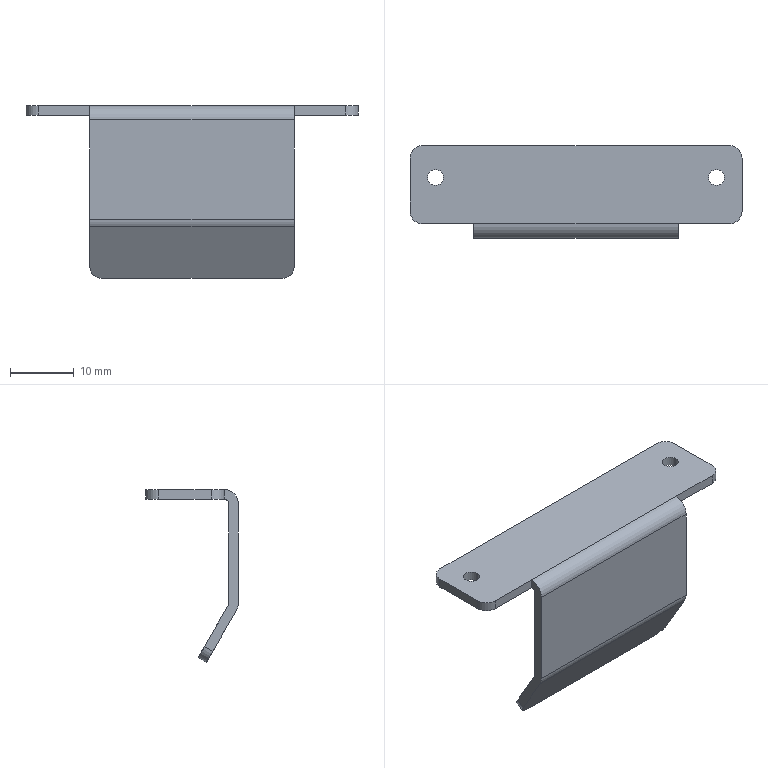Part | STEP file | 06-01-10 light source inclined plate A (Default) | 1 solid | 28 faces | box 52 x 14.5 x 27.062 mm | volume 2282 mm3 | cylinder 14 | plane 14 | commonest cylinder face diameters 4 x6 2.5 x4 1.473 x2 4.473 x2
STEP:
#1=CARTESIAN_POINT('',(20.75,1.5,0.));
#2=VERTEX_POINT('',#1);
#3=CARTESIAN_POINT('',(23.25,1.5,0.));
#4=VERTEX_POINT('',#3);
#5=CARTESIAN_POINT('',(22.,1.5,0.));
#6=DIRECTION('',(0.,0.,1.));
#7=DIRECTION('',(1.,0.,0.));
#8=AXIS2_PLACEMENT_3D('',#5,#6,#7);
#9=CIRCLE('',#8,1.25);
#10=EDGE_CURVE('',#2,#4,#9,.T.);
#11=ORIENTED_EDGE('',*,*,#10,.T.);
#12=CARTESIAN_POINT('',(23.25,1.5,-1.5));
#13=VERTEX_POINT('',#12);
#14=CARTESIAN_POINT('',(23.25,1.5,-1.5));
#15=DIRECTION('',(0.,0.,-1.));
#16=VECTOR('',#15,1000.);
#17=LINE('',#14,#16);
#18=EDGE_CURVE('',#4,#13,#17,.T.);
#19=ORIENTED_EDGE('',*,*,#18,.T.);
#20=CARTESIAN_POINT('',(20.75,1.5,-1.5));
#21=VERTEX_POINT('',#20);
#22=CARTESIAN_POINT('',(22.,1.5,-1.5));
#23=DIRECTION('',(0.,0.,-1.));
#24=DIRECTION('',(-1.,0.,0.));
#25=AXIS2_PLACEMENT_3D('',#22,#23,#24);
#26=CIRCLE('',#25,1.25);
#27=EDGE_CURVE('',#13,#21,#26,.T.);
#28=ORIENTED_EDGE('',*,*,#27,.T.);
#29=CARTESIAN_POINT('',(20.75,1.5,-1.5));
#30=DIRECTION('',(0.,0.,-1.));
#31=VECTOR('',#30,1000.);
#32=LINE('',#29,#31);
#33=EDGE_CURVE('',#2,#21,#32,.T.);
#34=ORIENTED_EDGE('',*,*,#33,.F.);
#35=EDGE_LOOP('',(#11,#19,#28,#34));
#36=FACE_OUTER_BOUND('',#35,.T.);
#37=CARTESIAN_POINT('',(22.,1.5,-1.5));
#38=DIRECTION('',(0.,0.,-1.));
#39=DIRECTION('',(-1.,0.,0.));
#40=AXIS2_PLACEMENT_3D('',#37,#38,#39);
#41=CYLINDRICAL_SURFACE('',#40,1.25);
#42=ADVANCED_FACE('',(#36),#41,.F.);
#43=CARTESIAN_POINT('',(-23.25,1.5,0.));
#44=VERTEX_POINT('',#43);
#45=CARTESIAN_POINT('',(-20.75,1.5,0.));
#46=VERTEX_POINT('',#45);
#47=CARTESIAN_POINT('',(-22.,1.5,0.));
#48=DIRECTION('',(0.,0.,1.));
#49=DIRECTION('',(1.,0.,0.));
#50=AXIS2_PLACEMENT_3D('',#47,#48,#49);
#51=CIRCLE('',#50,1.25);
#52=EDGE_CURVE('',#44,#46,#51,.T.);
#53=ORIENTED_EDGE('',*,*,#52,.T.);
#54=CARTESIAN_POINT('',(-20.75,1.5,-1.5));
#55=VERTEX_POINT('',#54);
#56=CARTESIAN_POINT('',(-20.75,1.5,-1.5));
#57=DIRECTION('',(0.,0.,-1.));
#58=VECTOR('',#57,1000.);
#59=LINE('',#56,#58);
#60=EDGE_CURVE('',#46,#55,#59,.T.);
#61=ORIENTED_EDGE('',*,*,#60,.T.);
#62=CARTESIAN_POINT('',(-23.25,1.5,-1.5));
#63=VERTEX_POINT('',#62);
#64=CARTESIAN_POINT('',(-22.,1.5,-1.5));
#65=DIRECTION('',(0.,0.,-1.));
#66=DIRECTION('',(-1.,0.,0.));
#67=AXIS2_PLACEMENT_3D('',#64,#65,#66);
#68=CIRCLE('',#67,1.25);
#69=EDGE_CURVE('',#55,#63,#68,.T.);
#70=ORIENTED_EDGE('',*,*,#69,.T.);
#71=CARTESIAN_POINT('',(-23.25,1.5,-1.5));
#72=DIRECTION('',(0.,0.,-1.));
#73=VECTOR('',#72,1000.);
#74=LINE('',#71,#73);
#75=EDGE_CURVE('',#44,#63,#74,.T.);
#76=ORIENTED_EDGE('',*,*,#75,.F.);
#77=EDGE_LOOP('',(#53,#61,#70,#76));
#78=FACE_OUTER_BOUND('',#77,.T.);
#79=CARTESIAN_POINT('',(-22.,1.5,-1.5));
#80=DIRECTION('',(0.,0.,-1.));
#81=DIRECTION('',(-1.,0.,0.));
#82=AXIS2_PLACEMENT_3D('',#79,#80,#81);
#83=CYLINDRICAL_SURFACE('',#82,1.25);
#84=ADVANCED_FACE('',(#78),#83,.F.);
#85=CARTESIAN_POINT('',(16.,-8.,-2.237));
#86=VERTEX_POINT('',#85);
#87=CARTESIAN_POINT('',(16.,-8.,-17.803));
#88=VERTEX_POINT('',#87);
#89=CARTESIAN_POINT('',(16.,-8.,-1.5));
#90=DIRECTION('',(0.,0.,-1.));
#91=VECTOR('',#90,1000.);
#92=LINE('',#89,#91);
#93=EDGE_CURVE('',#86,#88,#92,.T.);
#94=ORIENTED_EDGE('',*,*,#93,.F.);
#95=CARTESIAN_POINT('',(-16.,-8.,-2.237));
#96=VERTEX_POINT('',#95);
#97=CARTESIAN_POINT('',(-26.,-8.,-2.237));
#98=DIRECTION('',(-1.,0.,0.));
#99=VECTOR('',#98,1000.);
#100=LINE('',#97,#99);
#101=EDGE_CURVE('',#86,#96,#100,.T.);
#102=ORIENTED_EDGE('',*,*,#101,.T.);
#103=CARTESIAN_POINT('',(-16.,-8.,-17.803));
#104=VERTEX_POINT('',#103);
#105=CARTESIAN_POINT('',(-16.,-8.,-1.5));
#106=DIRECTION('',(0.,0.,1.));
#107=VECTOR('',#106,1000.);
#108=LINE('',#105,#107);
#109=EDGE_CURVE('',#104,#96,#108,.T.);
#110=ORIENTED_EDGE('',*,*,#109,.F.);
#111=CARTESIAN_POINT('',(-26.,-8.,-17.803));
#112=DIRECTION('',(1.,0.,0.));
#113=VECTOR('',#112,1000.);
#114=LINE('',#111,#113);
#115=EDGE_CURVE('',#104,#88,#114,.T.);
#116=ORIENTED_EDGE('',*,*,#115,.T.);
#117=EDGE_LOOP('',(#94,#102,#110,#116));
#118=FACE_OUTER_BOUND('',#117,.T.);
#119=CARTESIAN_POINT('',(-26.,-8.,-1.5));
#120=DIRECTION('',(0.,-1.,0.));
#121=DIRECTION('',(0.,0.,-1.));
#122=AXIS2_PLACEMENT_3D('',#119,#120,#121);
#123=PLANE('',#122);
#124=ADVANCED_FACE('',(#118),#123,.T.);
#125=CARTESIAN_POINT('',(16.,-6.5,-2.237));
#126=VERTEX_POINT('',#125);
#127=CARTESIAN_POINT('',(-16.,-6.5,-2.237));
#128=VERTEX_POINT('',#127);
#129=CARTESIAN_POINT('',(26.,-6.5,-2.237));
#130=DIRECTION('',(-1.,0.,0.));
#131=VECTOR('',#130,1000.);
#132=LINE('',#129,#131);
#133=EDGE_CURVE('',#126,#128,#132,.T.);
#134=ORIENTED_EDGE('',*,*,#133,.F.);
#135=CARTESIAN_POINT('',(16.,-6.5,-17.803));
#136=VERTEX_POINT('',#135);
#137=CARTESIAN_POINT('',(16.,-6.5,-1.5));
#138=DIRECTION('',(0.,0.,-1.));
#139=VECTOR('',#138,1000.);
#140=LINE('',#137,#139);
#141=EDGE_CURVE('',#126,#136,#140,.T.);
#142=ORIENTED_EDGE('',*,*,#141,.T.);
#143=CARTESIAN_POINT('',(-16.,-6.5,-17.803));
#144=VERTEX_POINT('',#143);
#145=CARTESIAN_POINT('',(-26.,-6.5,-17.803));
#146=DIRECTION('',(1.,0.,0.));
#147=VECTOR('',#146,1000.);
#148=LINE('',#145,#147);
#149=EDGE_CURVE('',#144,#136,#148,.T.);
#150=ORIENTED_EDGE('',*,*,#149,.F.);
#151=CARTESIAN_POINT('',(-16.,-6.5,-1.5));
#152=DIRECTION('',(0.,0.,1.));
#153=VECTOR('',#152,1000.);
#154=LINE('',#151,#153);
#155=EDGE_CURVE('',#144,#128,#154,.T.);
#156=ORIENTED_EDGE('',*,*,#155,.T.);
#157=EDGE_LOOP('',(#134,#142,#150,#156));
#158=FACE_OUTER_BOUND('',#157,.T.);
#159=CARTESIAN_POINT('',(-26.,-6.5,-1.5));
#160=DIRECTION('',(0.,-1.,0.));
#161=DIRECTION('',(0.,0.,-1.));
#162=AXIS2_PLACEMENT_3D('',#159,#160,#161);
#163=PLANE('',#162);
#164=ADVANCED_FACE('',(#158),#163,.F.);
#165=CARTESIAN_POINT('',(-26.,4.5,-1.5));
#166=VERTEX_POINT('',#165);
#167=CARTESIAN_POINT('',(-26.,-3.763,-1.5));
#168=VERTEX_POINT('',#167);
#169=CARTESIAN_POINT('',(-26.,6.5,-1.5));
#170=DIRECTION('',(0.,-1.,0.));
#171=VECTOR('',#170,1000.);
#172=LINE('',#169,#171);
#173=EDGE_CURVE('',#166,#168,#172,.T.);
#174=ORIENTED_EDGE('',*,*,#173,.T.);
#175=CARTESIAN_POINT('',(-26.,-3.763,0.));
#176=VERTEX_POINT('',#175);
#177=CARTESIAN_POINT('',(-26.,-3.763,0.));
#178=DIRECTION('',(0.,0.,1.));
#179=VECTOR('',#178,1000.);
#180=LINE('',#177,#179);
#181=EDGE_CURVE('',#168,#176,#180,.T.);
#182=ORIENTED_EDGE('',*,*,#181,.T.);
#183=CARTESIAN_POINT('',(-26.,4.5,0.));
#184=VERTEX_POINT('',#183);
#185=CARTESIAN_POINT('',(-26.,6.5,0.));
#186=DIRECTION('',(0.,-1.,0.));
#187=VECTOR('',#186,1000.);
#188=LINE('',#185,#187);
#189=EDGE_CURVE('',#184,#176,#188,.T.);
#190=ORIENTED_EDGE('',*,*,#189,.F.);
#191=CARTESIAN_POINT('',(-26.,4.5,-1.5));
#192=DIRECTION('',(0.,0.,-1.));
#193=VECTOR('',#192,1000.);
#194=LINE('',#191,#193);
#195=EDGE_CURVE('',#184,#166,#194,.T.);
#196=ORIENTED_EDGE('',*,*,#195,.T.);
#197=EDGE_LOOP('',(#174,#182,#190,#196));
#198=FACE_OUTER_BOUND('',#197,.T.);
#199=CARTESIAN_POINT('',(-26.,6.5,-1.5));
#200=DIRECTION('',(-1.,0.,0.));
#201=DIRECTION('',(0.,0.,1.));
#202=AXIS2_PLACEMENT_3D('',#199,#200,#201);
#203=PLANE('',#202);
#204=ADVANCED_FACE('',(#198),#203,.T.);
#205=CARTESIAN_POINT('',(22.,1.5,-1.5));
#206=DIRECTION('',(0.,0.,-1.));
#207=DIRECTION('',(-1.,0.,0.));
#208=AXIS2_PLACEMENT_3D('',#205,#206,#207);
#209=CIRCLE('',#208,1.25);
#210=EDGE_CURVE('',#21,#13,#209,.T.);
#211=ORIENTED_EDGE('',*,*,#210,.F.);
#212=ORIENTED_EDGE('',*,*,#27,.F.);
#213=EDGE_LOOP('',(#211,#212));
#214=FACE_BOUND('',#213,.T.);
#215=CARTESIAN_POINT('',(-22.,1.5,-1.5));
#216=DIRECTION('',(0.,0.,-1.));
#217=DIRECTION('',(-1.,0.,0.));
#218=AXIS2_PLACEMENT_3D('',#215,#216,#217);
#219=CIRCLE('',#218,1.25);
#220=EDGE_CURVE('',#63,#55,#219,.T.);
#221=ORIENTED_EDGE('',*,*,#220,.F.);
#222=ORIENTED_EDGE('',*,*,#69,.F.);
#223=EDGE_LOOP('',(#221,#222));
#224=FACE_BOUND('',#223,.T.);
#225=CARTESIAN_POINT('',(-24.,-5.763,-1.5));
#226=VERTEX_POINT('',#225);
#227=CARTESIAN_POINT('',(-16.,-5.763,-1.5));
#228=VERTEX_POINT('',#227);
#229=CARTESIAN_POINT('',(-26.,-5.763,-1.5));
#230=DIRECTION('',(1.,0.,0.));
#231=VECTOR('',#230,1000.);
#232=LINE('',#229,#231);
#233=EDGE_CURVE('',#226,#228,#232,.T.);
#234=ORIENTED_EDGE('',*,*,#233,.F.);
#235=CARTESIAN_POINT('',(-24.,-3.763,-1.5));
#236=DIRECTION('',(0.,0.,-1.));
#237=DIRECTION('',(1.,0.,0.));
#238=AXIS2_PLACEMENT_3D('',#235,#236,#237);
#239=CIRCLE('',#238,2.);
#240=EDGE_CURVE('',#226,#168,#239,.T.);
#241=ORIENTED_EDGE('',*,*,#240,.T.);
#242=ORIENTED_EDGE('',*,*,#173,.F.);
#243=CARTESIAN_POINT('',(-24.,6.5,-1.5));
#244=VERTEX_POINT('',#243);
#245=CARTESIAN_POINT('',(-24.,4.5,-1.5));
#246=DIRECTION('',(0.,0.,-1.));
#247=DIRECTION('',(1.,0.,0.));
#248=AXIS2_PLACEMENT_3D('',#245,#246,#247);
#249=CIRCLE('',#248,2.);
#250=EDGE_CURVE('',#166,#244,#249,.T.);
#251=ORIENTED_EDGE('',*,*,#250,.T.);
#252=CARTESIAN_POINT('',(24.,6.5,-1.5));
#253=VERTEX_POINT('',#252);
#254=CARTESIAN_POINT('',(-26.,6.5,-1.5));
#255=DIRECTION('',(-1.,0.,0.));
#256=VECTOR('',#255,1000.);
#257=LINE('',#254,#256);
#258=EDGE_CURVE('',#253,#244,#257,.T.);
#259=ORIENTED_EDGE('',*,*,#258,.F.);
#260=CARTESIAN_POINT('',(26.,4.5,-1.5));
#261=VERTEX_POINT('',#260);
#262=CARTESIAN_POINT('',(24.,4.5,-1.5));
#263=DIRECTION('',(0.,0.,-1.));
#264=DIRECTION('',(1.,0.,0.));
#265=AXIS2_PLACEMENT_3D('',#262,#263,#264);
#266=CIRCLE('',#265,2.);
#267=EDGE_CURVE('',#253,#261,#266,.T.);
#268=ORIENTED_EDGE('',*,*,#267,.T.);
#269=CARTESIAN_POINT('',(26.,-3.763,-1.5));
#270=VERTEX_POINT('',#269);
#271=CARTESIAN_POINT('',(26.,6.5,-1.5));
#272=DIRECTION('',(0.,1.,0.));
#273=VECTOR('',#272,1000.);
#274=LINE('',#271,#273);
#275=EDGE_CURVE('',#270,#261,#274,.T.);
#276=ORIENTED_EDGE('',*,*,#275,.F.);
#277=CARTESIAN_POINT('',(24.,-5.763,-1.5));
#278=VERTEX_POINT('',#277);
#279=CARTESIAN_POINT('',(24.,-3.763,-1.5));
#280=DIRECTION('',(0.,0.,-1.));
#281=DIRECTION('',(1.,0.,0.));
#282=AXIS2_PLACEMENT_3D('',#279,#280,#281);
#283=CIRCLE('',#282,2.);
#284=EDGE_CURVE('',#270,#278,#283,.T.);
#285=ORIENTED_EDGE('',*,*,#284,.T.);
#286=CARTESIAN_POINT('',(16.,-5.763,-1.5));
#287=VERTEX_POINT('',#286);
#288=CARTESIAN_POINT('',(-26.,-5.763,-1.5));
#289=DIRECTION('',(1.,0.,0.));
#290=VECTOR('',#289,1000.);
#291=LINE('',#288,#290);
#292=EDGE_CURVE('',#287,#278,#291,.T.);
#293=ORIENTED_EDGE('',*,*,#292,.F.);
#294=CARTESIAN_POINT('',(-26.,-5.763,-1.5));
#295=DIRECTION('',(1.,0.,0.));
#296=VECTOR('',#295,1000.);
#297=LINE('',#294,#296);
#298=EDGE_CURVE('',#228,#287,#297,.T.);
#299=ORIENTED_EDGE('',*,*,#298,.F.);
#300=EDGE_LOOP('',(#234,#241,#242,#251,#259,#268,#276,#285,#293,#299));
#301=FACE_OUTER_BOUND('',#300,.T.);
#302=CARTESIAN_POINT('',(26.,-6.5,-1.5));
#303=DIRECTION('',(0.,0.,1.));
#304=DIRECTION('',(1.,0.,0.));
#305=AXIS2_PLACEMENT_3D('',#302,#303,#304);
#306=PLANE('',#305);
#307=ADVANCED_FACE('',(#214,#224,#301),#306,.F.);
#308=ORIENTED_EDGE('',*,*,#10,.F.);
#309=CARTESIAN_POINT('',(22.,1.5,0.));
#310=DIRECTION('',(0.,0.,1.));
#311=DIRECTION('',(1.,0.,0.));
#312=AXIS2_PLACEMENT_3D('',#309,#310,#311);
#313=CIRCLE('',#312,1.25);
#314=EDGE_CURVE('',#4,#2,#313,.T.);
#315=ORIENTED_EDGE('',*,*,#314,.F.);
#316=EDGE_LOOP('',(#308,#315));
#317=FACE_BOUND('',#316,.T.);
#318=ORIENTED_EDGE('',*,*,#52,.F.);
#319=CARTESIAN_POINT('',(-22.,1.5,0.));
#320=DIRECTION('',(0.,0.,1.));
#321=DIRECTION('',(1.,0.,0.));
#322=AXIS2_PLACEMENT_3D('',#319,#320,#321);
#323=CIRCLE('',#322,1.25);
#324=EDGE_CURVE('',#46,#44,#323,.T.);
#325=ORIENTED_EDGE('',*,*,#324,.F.);
#326=EDGE_LOOP('',(#318,#325));
#327=FACE_BOUND('',#326,.T.);
#328=ORIENTED_EDGE('',*,*,#189,.T.);
#329=CARTESIAN_POINT('',(-24.,-5.763,0.));
#330=VERTEX_POINT('',#329);
#331=CARTESIAN_POINT('',(-24.,-3.763,0.));
#332=DIRECTION('',(0.,0.,1.));
#333=DIRECTION('',(1.,0.,0.));
#334=AXIS2_PLACEMENT_3D('',#331,#332,#333);
#335=CIRCLE('',#334,2.);
#336=EDGE_CURVE('',#176,#330,#335,.T.);
#337=ORIENTED_EDGE('',*,*,#336,.T.);
#338=CARTESIAN_POINT('',(-16.,-5.763,0.));
#339=VERTEX_POINT('',#338);
#340=CARTESIAN_POINT('',(-26.,-5.763,0.));
#341=DIRECTION('',(1.,0.,0.));
#342=VECTOR('',#341,1000.);
#343=LINE('',#340,#342);
#344=EDGE_CURVE('',#330,#339,#343,.T.);
#345=ORIENTED_EDGE('',*,*,#344,.T.);
#346=CARTESIAN_POINT('',(16.,-5.763,0.));
#347=VERTEX_POINT('',#346);
#348=CARTESIAN_POINT('',(-26.,-5.763,0.));
#349=DIRECTION('',(1.,0.,0.));
#350=VECTOR('',#349,1000.);
#351=LINE('',#348,#350);
#352=EDGE_CURVE('',#339,#347,#351,.T.);
#353=ORIENTED_EDGE('',*,*,#352,.T.);
#354=CARTESIAN_POINT('',(24.,-5.763,0.));
#355=VERTEX_POINT('',#354);
#356=CARTESIAN_POINT('',(16.,-5.763,0.));
#357=DIRECTION('',(1.,0.,0.));
#358=VECTOR('',#357,1000.);
#359=LINE('',#356,#358);
#360=EDGE_CURVE('',#347,#355,#359,.T.);
#361=ORIENTED_EDGE('',*,*,#360,.T.);
#362=CARTESIAN_POINT('',(26.,-3.763,0.));
#363=VERTEX_POINT('',#362);
#364=CARTESIAN_POINT('',(24.,-3.763,0.));
#365=DIRECTION('',(0.,0.,1.));
#366=DIRECTION('',(1.,0.,0.));
#367=AXIS2_PLACEMENT_3D('',#364,#365,#366);
#368=CIRCLE('',#367,2.);
#369=EDGE_CURVE('',#355,#363,#368,.T.);
#370=ORIENTED_EDGE('',*,*,#369,.T.);
#371=CARTESIAN_POINT('',(26.,4.5,0.));
#372=VERTEX_POINT('',#371);
#373=CARTESIAN_POINT('',(26.,6.5,0.));
#374=DIRECTION('',(0.,1.,0.));
#375=VECTOR('',#374,1000.);
#376=LINE('',#373,#375);
#377=EDGE_CURVE('',#363,#372,#376,.T.);
#378=ORIENTED_EDGE('',*,*,#377,.T.);
#379=CARTESIAN_POINT('',(24.,6.5,0.));
#380=VERTEX_POINT('',#379);
#381=CARTESIAN_POINT('',(24.,4.5,0.));
#382=DIRECTION('',(0.,0.,1.));
#383=DIRECTION('',(1.,0.,0.));
#384=AXIS2_PLACEMENT_3D('',#381,#382,#383);
#385=CIRCLE('',#384,2.);
#386=EDGE_CURVE('',#372,#380,#385,.T.);
#387=ORIENTED_EDGE('',*,*,#386,.T.);
#388=CARTESIAN_POINT('',(-24.,6.5,0.));
#389=VERTEX_POINT('',#388);
#390=CARTESIAN_POINT('',(-26.,6.5,0.));
#391=DIRECTION('',(-1.,0.,0.));
#392=VECTOR('',#391,1000.);
#393=LINE('',#390,#392);
#394=EDGE_CURVE('',#380,#389,#393,.T.);
#395=ORIENTED_EDGE('',*,*,#394,.T.);
#396=CARTESIAN_POINT('',(-24.,4.5,0.));
#397=DIRECTION('',(0.,0.,1.));
#398=DIRECTION('',(1.,0.,0.));
#399=AXIS2_PLACEMENT_3D('',#396,#397,#398);
#400=CIRCLE('',#399,2.);
#401=EDGE_CURVE('',#389,#184,#400,.T.);
#402=ORIENTED_EDGE('',*,*,#401,.T.);
#403=EDGE_LOOP('',(#328,#337,#345,#353,#361,#370,#378,#387,#395,#402));
#404=FACE_OUTER_BOUND('',#403,.T.);
#405=CARTESIAN_POINT('',(26.,-6.5,0.));
#406=DIRECTION('',(0.,0.,1.));
#407=DIRECTION('',(1.,0.,0.));
#408=AXIS2_PLACEMENT_3D('',#405,#406,#407);
#409=PLANE('',#408);
#410=ADVANCED_FACE('',(#317,#327,#404),#409,.T.);
#411=ORIENTED_EDGE('',*,*,#275,.T.);
#412=CARTESIAN_POINT('',(26.,4.5,-1.5));
#413=DIRECTION('',(0.,0.,1.));
#414=VECTOR('',#413,1000.);
#415=LINE('',#412,#414);
#416=EDGE_CURVE('',#261,#372,#415,.T.);
#417=ORIENTED_EDGE('',*,*,#416,.T.);
#418=ORIENTED_EDGE('',*,*,#377,.F.);
#419=CARTESIAN_POINT('',(26.,-3.763,-1.5));
#420=DIRECTION('',(0.,0.,-1.));
#421=VECTOR('',#420,1000.);
#422=LINE('',#419,#421);
#423=EDGE_CURVE('',#363,#270,#422,.T.);
#424=ORIENTED_EDGE('',*,*,#423,.T.);
#425=EDGE_LOOP('',(#411,#417,#418,#424));
#426=FACE_OUTER_BOUND('',#425,.T.);
#427=CARTESIAN_POINT('',(26.,6.5,-1.5));
#428=DIRECTION('',(1.,0.,0.));
#429=DIRECTION('',(0.,0.,-1.));
#430=AXIS2_PLACEMENT_3D('',#427,#428,#429);
#431=PLANE('',#430);
#432=ADVANCED_FACE('',(#426),#431,.T.);
#433=ORIENTED_EDGE('',*,*,#258,.T.);
#434=CARTESIAN_POINT('',(-24.,6.5,-1.5));
#435=DIRECTION('',(0.,0.,1.));
#436=VECTOR('',#435,1000.);
#437=LINE('',#434,#436);
#438=EDGE_CURVE('',#244,#389,#437,.T.);
#439=ORIENTED_EDGE('',*,*,#438,.T.);
#440=ORIENTED_EDGE('',*,*,#394,.F.);
#441=CARTESIAN_POINT('',(24.,6.5,-1.5));
#442=DIRECTION('',(0.,0.,-1.));
#443=VECTOR('',#442,1000.);
#444=LINE('',#441,#443);
#445=EDGE_CURVE('',#380,#253,#444,.T.);
#446=ORIENTED_EDGE('',*,*,#445,.T.);
#447=EDGE_LOOP('',(#433,#439,#440,#446));
#448=FACE_OUTER_BOUND('',#447,.T.);
#449=CARTESIAN_POINT('',(-26.,6.5,-1.5));
#450=DIRECTION('',(0.,1.,0.));
#451=DIRECTION('',(0.,0.,1.));
#452=AXIS2_PLACEMENT_3D('',#449,#450,#451);
#453=PLANE('',#452);
#454=ADVANCED_FACE('',(#448),#453,.T.);
#455=CARTESIAN_POINT('',(16.,-5.763,-2.237));
#456=DIRECTION('',(1.,0.,0.));
#457=DIRECTION('',(0.,0.,1.));
#458=AXIS2_PLACEMENT_3D('',#455,#456,#457);
#459=CIRCLE('',#458,2.237);
#460=EDGE_CURVE('',#347,#86,#459,.T.);
#461=ORIENTED_EDGE('',*,*,#460,.F.);
#462=ORIENTED_EDGE('',*,*,#352,.F.);
#463=CARTESIAN_POINT('',(-16.,-5.763,-2.237));
#464=DIRECTION('',(-1.,0.,0.));
#465=DIRECTION('',(0.,0.,-1.));
#466=AXIS2_PLACEMENT_3D('',#463,#464,#465);
#467=CIRCLE('',#466,2.237);
#468=EDGE_CURVE('',#96,#339,#467,.T.);
#469=ORIENTED_EDGE('',*,*,#468,.F.);
#470=ORIENTED_EDGE('',*,*,#101,.F.);
#471=EDGE_LOOP('',(#461,#462,#469,#470));
#472=FACE_OUTER_BOUND('',#471,.T.);
#473=CARTESIAN_POINT('',(-26.,-5.763,-2.237));
#474=DIRECTION('',(-1.,0.,0.));
#475=DIRECTION('',(0.,-1.,0.));
#476=AXIS2_PLACEMENT_3D('',#473,#474,#475);
#477=CYLINDRICAL_SURFACE('',#476,2.237);
#478=ADVANCED_FACE('',(#472),#477,.T.);
#479=ORIENTED_EDGE('',*,*,#298,.T.);
#480=CARTESIAN_POINT('',(16.,-5.763,-2.237));
#481=DIRECTION('',(1.,0.,0.));
#482=DIRECTION('',(0.,0.,1.));
#483=AXIS2_PLACEMENT_3D('',#480,#481,#482);
#484=CIRCLE('',#483,0.7366);
#485=EDGE_CURVE('',#287,#126,#484,.T.);
#486=ORIENTED_EDGE('',*,*,#485,.T.);
#487=ORIENTED_EDGE('',*,*,#133,.T.);
#488=CARTESIAN_POINT('',(-16.,-5.763,-2.237));
#489=DIRECTION('',(-1.,0.,0.));
#490=DIRECTION('',(0.,0.,-1.));
#491=AXIS2_PLACEMENT_3D('',#488,#489,#490);
#492=CIRCLE('',#491,0.7366);
#493=EDGE_CURVE('',#128,#228,#492,.T.);
#494=ORIENTED_EDGE('',*,*,#493,.T.);
#495=EDGE_LOOP('',(#479,#486,#487,#494));
#496=FACE_OUTER_BOUND('',#495,.T.);
#497=CARTESIAN_POINT('',(-26.,-5.763,-2.237));
#498=DIRECTION('',(-1.,0.,0.));
#499=DIRECTION('',(0.,-1.,0.));
#500=AXIS2_PLACEMENT_3D('',#497,#498,#499);
#501=CYLINDRICAL_SURFACE('',#500,0.7366);
#502=ADVANCED_FACE('',(#496),#501,.F.);
#503=ORIENTED_EDGE('',*,*,#60,.F.);
#504=ORIENTED_EDGE('',*,*,#324,.T.);
#505=ORIENTED_EDGE('',*,*,#75,.T.);
#506=ORIENTED_EDGE('',*,*,#220,.T.);
#507=EDGE_LOOP('',(#503,#504,#505,#506));
#508=FACE_OUTER_BOUND('',#507,.T.);
#509=CARTESIAN_POINT('',(-22.,1.5,-1.5));
#510=DIRECTION('',(0.,0.,-1.));
#511=DIRECTION('',(-1.,0.,0.));
#512=AXIS2_PLACEMENT_3D('',#509,#510,#511);
#513=CYLINDRICAL_SURFACE('',#512,1.25);
#514=ADVANCED_FACE('',(#508),#513,.F.);
#515=ORIENTED_EDGE('',*,*,#18,.F.);
#516=ORIENTED_EDGE('',*,*,#314,.T.);
#517=ORIENTED_EDGE('',*,*,#33,.T.);
#518=ORIENTED_EDGE('',*,*,#210,.T.);
#519=EDGE_LOOP('',(#515,#516,#517,#518));
#520=FACE_OUTER_BOUND('',#519,.T.);
#521=CARTESIAN_POINT('',(22.,1.5,-1.5));
#522=DIRECTION('',(0.,0.,-1.));
#523=DIRECTION('',(-1.,0.,0.));
#524=AXIS2_PLACEMENT_3D('',#521,#522,#523);
#525=CYLINDRICAL_SURFACE('',#524,1.25);
#526=ADVANCED_FACE('',(#520),#525,.F.);
#527=CARTESIAN_POINT('',(16.,-7.7,-18.921));
#528=VERTEX_POINT('',#527);
#529=CARTESIAN_POINT('',(16.,-5.763,-17.803));
#530=DIRECTION('',(1.,0.,0.));
#531=DIRECTION('',(0.,0.,1.));
#532=AXIS2_PLACEMENT_3D('',#529,#530,#531);
#533=CIRCLE('',#532,2.237);
#534=EDGE_CURVE('',#88,#528,#533,.T.);
#535=ORIENTED_EDGE('',*,*,#534,.F.);
#536=ORIENTED_EDGE('',*,*,#115,.F.);
#537=CARTESIAN_POINT('',(-16.,-7.7,-18.921));
#538=VERTEX_POINT('',#537);
#539=CARTESIAN_POINT('',(-16.,-5.763,-17.803));
#540=DIRECTION('',(-1.,0.,0.));
#541=DIRECTION('',(0.,0.,-1.));
#542=AXIS2_PLACEMENT_3D('',#539,#540,#541);
#543=CIRCLE('',#542,2.237);
#544=EDGE_CURVE('',#538,#104,#543,.T.);
#545=ORIENTED_EDGE('',*,*,#544,.F.);
#546=CARTESIAN_POINT('',(-26.,-7.7,-18.921));
#547=DIRECTION('',(-1.,0.,0.));
#548=VECTOR('',#547,1000.);
#549=LINE('',#546,#548);
#550=EDGE_CURVE('',#528,#538,#549,.T.);
#551=ORIENTED_EDGE('',*,*,#550,.F.);
#552=EDGE_LOOP('',(#535,#536,#545,#551));
#553=FACE_OUTER_BOUND('',#552,.T.);
#554=CARTESIAN_POINT('',(-26.,-5.763,-17.803));
#555=DIRECTION('',(-1.,0.,0.));
#556=DIRECTION('',(0.,-0.866,-0.5));
#557=AXIS2_PLACEMENT_3D('',#554,#555,#556);
#558=CYLINDRICAL_SURFACE('',#557,2.237);
#559=ADVANCED_FACE('',(#553),#558,.T.);
#560=ORIENTED_EDGE('',*,*,#149,.T.);
#561=CARTESIAN_POINT('',(16.,-6.401,-18.171));
#562=VERTEX_POINT('',#561);
#563=CARTESIAN_POINT('',(16.,-5.763,-17.803));
#564=DIRECTION('',(1.,0.,0.));
#565=DIRECTION('',(0.,0.,1.));
#566=AXIS2_PLACEMENT_3D('',#563,#564,#565);
#567=CIRCLE('',#566,0.7366);
#568=EDGE_CURVE('',#136,#562,#567,.T.);
#569=ORIENTED_EDGE('',*,*,#568,.T.);
#570=CARTESIAN_POINT('',(-16.,-6.401,-18.171));
#571=VERTEX_POINT('',#570);
#572=CARTESIAN_POINT('',(26.,-6.401,-18.171));
#573=DIRECTION('',(-1.,0.,0.));
#574=VECTOR('',#573,1000.);
#575=LINE('',#572,#574);
#576=EDGE_CURVE('',#562,#571,#575,.T.);
#577=ORIENTED_EDGE('',*,*,#576,.T.);
#578=CARTESIAN_POINT('',(-16.,-5.763,-17.803));
#579=DIRECTION('',(-1.,0.,0.));
#580=DIRECTION('',(0.,0.,-1.));
#581=AXIS2_PLACEMENT_3D('',#578,#579,#580);
#582=CIRCLE('',#581,0.7366);
#583=EDGE_CURVE('',#571,#144,#582,.T.);
#584=ORIENTED_EDGE('',*,*,#583,.T.);
#585=EDGE_LOOP('',(#560,#569,#577,#584));
#586=FACE_OUTER_BOUND('',#585,.T.);
#587=CARTESIAN_POINT('',(-26.,-5.763,-17.803));
#588=DIRECTION('',(-1.,0.,0.));
#589=DIRECTION('',(0.,-0.866,-0.5));
#590=AXIS2_PLACEMENT_3D('',#587,#588,#589);
#591=CYLINDRICAL_SURFACE('',#590,0.7366);
#592=ADVANCED_FACE('',(#586),#591,.F.);
#593=CARTESIAN_POINT('',(14.,-3.,-27.062));
#594=VERTEX_POINT('',#593);
#595=CARTESIAN_POINT('',(-14.,-3.,-27.062));
#596=VERTEX_POINT('',#595);
#597=CARTESIAN_POINT('',(-26.,-3.,-27.062));
#598=DIRECTION('',(-1.,0.,0.));
#599=VECTOR('',#598,1000.);
#600=LINE('',#597,#599);
#601=EDGE_CURVE('',#594,#596,#600,.T.);
#602=ORIENTED_EDGE('',*,*,#601,.F.);
#603=CARTESIAN_POINT('',(16.,-4.,-25.33));
#604=VERTEX_POINT('',#603);
#605=CARTESIAN_POINT('',(14.,-4.,-25.33));
#606=DIRECTION('',(0.,-0.866,-0.5));
#607=DIRECTION('',(0.,0.5,-0.866));
#608=AXIS2_PLACEMENT_3D('',#605,#606,#607);
#609=CIRCLE('',#608,2.);
#610=EDGE_CURVE('',#594,#604,#609,.T.);
#611=ORIENTED_EDGE('',*,*,#610,.T.);
#612=CARTESIAN_POINT('',(16.,-7.799,-18.75));
#613=DIRECTION('',(0.,0.5,-0.866));
#614=VECTOR('',#613,1000.);
#615=LINE('',#612,#614);
#616=EDGE_CURVE('',#528,#604,#615,.T.);
#617=ORIENTED_EDGE('',*,*,#616,.F.);
#618=ORIENTED_EDGE('',*,*,#550,.T.);
#619=CARTESIAN_POINT('',(-16.,-4.,-25.33));
#620=VERTEX_POINT('',#619);
#621=CARTESIAN_POINT('',(-16.,-7.799,-18.75));
#622=DIRECTION('',(0.,-0.5,0.866));
#623=VECTOR('',#622,1000.);
#624=LINE('',#621,#623);
#625=EDGE_CURVE('',#620,#538,#624,.T.);
#626=ORIENTED_EDGE('',*,*,#625,.F.);
#627=CARTESIAN_POINT('',(-14.,-4.,-25.33));
#628=DIRECTION('',(0.,-0.866,-0.5));
#629=DIRECTION('',(0.,0.5,-0.866));
#630=AXIS2_PLACEMENT_3D('',#627,#628,#629);
#631=CIRCLE('',#630,2.);
#632=EDGE_CURVE('',#620,#596,#631,.T.);
#633=ORIENTED_EDGE('',*,*,#632,.T.);
#634=EDGE_LOOP('',(#602,#611,#617,#618,#626,#633));
#635=FACE_OUTER_BOUND('',#634,.T.);
#636=CARTESIAN_POINT('',(-26.,-7.799,-18.75));
#637=DIRECTION('',(0.,-0.866,-0.5));
#638=DIRECTION('',(0.,0.5,-0.866));
#639=AXIS2_PLACEMENT_3D('',#636,#637,#638);
#640=PLANE('',#639);
#641=ADVANCED_FACE('',(#635),#640,.T.);
#642=CARTESIAN_POINT('',(16.,-2.701,-24.58));
#643=VERTEX_POINT('',#642);
#644=CARTESIAN_POINT('',(16.,-6.5,-18.));
#645=DIRECTION('',(0.,0.5,-0.866));
#646=VECTOR('',#645,1000.);
#647=LINE('',#644,#646);
#648=EDGE_CURVE('',#562,#643,#647,.T.);
#649=ORIENTED_EDGE('',*,*,#648,.T.);
#650=CARTESIAN_POINT('',(14.,-1.701,-26.312));
#651=VERTEX_POINT('',#650);
#652=CARTESIAN_POINT('',(14.,-2.701,-24.58));
#653=DIRECTION('',(0.,0.866,0.5));
#654=DIRECTION('',(0.,0.5,-0.866));
#655=AXIS2_PLACEMENT_3D('',#652,#653,#654);
#656=CIRCLE('',#655,2.);
#657=EDGE_CURVE('',#643,#651,#656,.T.);
#658=ORIENTED_EDGE('',*,*,#657,.T.);
#659=CARTESIAN_POINT('',(-14.,-1.701,-26.312));
#660=VERTEX_POINT('',#659);
#661=CARTESIAN_POINT('',(-26.,-1.701,-26.312));
#662=DIRECTION('',(-1.,0.,0.));
#663=VECTOR('',#662,1000.);
#664=LINE('',#661,#663);
#665=EDGE_CURVE('',#651,#660,#664,.T.);
#666=ORIENTED_EDGE('',*,*,#665,.T.);
#667=CARTESIAN_POINT('',(-16.,-2.701,-24.58));
#668=VERTEX_POINT('',#667);
#669=CARTESIAN_POINT('',(-14.,-2.701,-24.58));
#670=DIRECTION('',(0.,0.866,0.5));
#671=DIRECTION('',(0.,0.5,-0.866));
#672=AXIS2_PLACEMENT_3D('',#669,#670,#671);
#673=CIRCLE('',#672,2.);
#674=EDGE_CURVE('',#660,#668,#673,.T.);
#675=ORIENTED_EDGE('',*,*,#674,.T.);
#676=CARTESIAN_POINT('',(-16.,-6.5,-18.));
#677=DIRECTION('',(0.,-0.5,0.866));
#678=VECTOR('',#677,1000.);
#679=LINE('',#676,#678);
#680=EDGE_CURVE('',#668,#571,#679,.T.);
#681=ORIENTED_EDGE('',*,*,#680,.T.);
#682=ORIENTED_EDGE('',*,*,#576,.F.);
#683=EDGE_LOOP('',(#649,#658,#666,#675,#681,#682));
#684=FACE_OUTER_BOUND('',#683,.T.);
#685=CARTESIAN_POINT('',(-26.,-6.5,-18.));
#686=DIRECTION('',(0.,-0.866,-0.5));
#687=DIRECTION('',(0.,0.5,-0.866));
#688=AXIS2_PLACEMENT_3D('',#685,#686,#687);
#689=PLANE('',#688);
#690=ADVANCED_FACE('',(#684),#689,.F.);
#691=ORIENTED_EDGE('',*,*,#665,.F.);
#692=CARTESIAN_POINT('',(14.,-3.,-27.062));
#693=DIRECTION('',(0.,-0.866,-0.5));
#694=VECTOR('',#693,1000.);
#695=LINE('',#692,#694);
#696=EDGE_CURVE('',#651,#594,#695,.T.);
#697=ORIENTED_EDGE('',*,*,#696,.T.);
#698=ORIENTED_EDGE('',*,*,#601,.T.);
#699=CARTESIAN_POINT('',(-14.,-1.701,-26.312));
#700=DIRECTION('',(0.,0.866,0.5));
#701=VECTOR('',#700,1000.);
#702=LINE('',#699,#701);
#703=EDGE_CURVE('',#596,#660,#702,.T.);
#704=ORIENTED_EDGE('',*,*,#703,.T.);
#705=EDGE_LOOP('',(#691,#697,#698,#704));
#706=FACE_OUTER_BOUND('',#705,.T.);
#707=CARTESIAN_POINT('',(-26.,-3.,-27.062));
#708=DIRECTION('',(0.,0.5,-0.866));
#709=DIRECTION('',(0.,0.866,0.5));
#710=AXIS2_PLACEMENT_3D('',#707,#708,#709);
#711=PLANE('',#710);
#712=ADVANCED_FACE('',(#706),#711,.T.);
#713=ORIENTED_EDGE('',*,*,#344,.F.);
#714=CARTESIAN_POINT('',(-24.,-5.763,-1.5));
#715=DIRECTION('',(0.,0.,-1.));
#716=VECTOR('',#715,1000.);
#717=LINE('',#714,#716);
#718=EDGE_CURVE('',#330,#226,#717,.T.);
#719=ORIENTED_EDGE('',*,*,#718,.T.);
#720=ORIENTED_EDGE('',*,*,#233,.T.);
#721=CARTESIAN_POINT('',(-16.,-5.763,0.));
#722=DIRECTION('',(0.,0.,-1.));
#723=VECTOR('',#722,1000.);
#724=LINE('',#721,#723);
#725=EDGE_CURVE('',#339,#228,#724,.T.);
#726=ORIENTED_EDGE('',*,*,#725,.F.);
#727=EDGE_LOOP('',(#713,#719,#720,#726));
#728=FACE_OUTER_BOUND('',#727,.T.);
#729=CARTESIAN_POINT('',(-16.,-5.763,0.));
#730=DIRECTION('',(0.,1.,0.));
#731=DIRECTION('',(0.,0.,1.));
#732=AXIS2_PLACEMENT_3D('',#729,#730,#731);
#733=PLANE('',#732);
#734=ADVANCED_FACE('',(#728),#733,.F.);
#735=ORIENTED_EDGE('',*,*,#680,.F.);
#736=CARTESIAN_POINT('',(-16.,-4.,-25.33));
#737=DIRECTION('',(0.,-0.866,-0.5));
#738=VECTOR('',#737,1000.);
#739=LINE('',#736,#738);
#740=EDGE_CURVE('',#668,#620,#739,.T.);
#741=ORIENTED_EDGE('',*,*,#740,.T.);
#742=ORIENTED_EDGE('',*,*,#625,.T.);
#743=ORIENTED_EDGE('',*,*,#544,.T.);
#744=ORIENTED_EDGE('',*,*,#109,.T.);
#745=ORIENTED_EDGE('',*,*,#468,.T.);
#746=ORIENTED_EDGE('',*,*,#725,.T.);
#747=ORIENTED_EDGE('',*,*,#493,.F.);
#748=ORIENTED_EDGE('',*,*,#155,.F.);
#749=ORIENTED_EDGE('',*,*,#583,.F.);
#750=EDGE_LOOP('',(#735,#741,#742,#743,#744,#745,#746,#747,#748,#749));
#751=FACE_OUTER_BOUND('',#750,.T.);
#752=CARTESIAN_POINT('',(-16.,-10.705,0.));
#753=DIRECTION('',(1.,0.,0.));
#754=DIRECTION('',(0.,0.,-1.));
#755=AXIS2_PLACEMENT_3D('',#752,#753,#754);
#756=PLANE('',#755);
#757=ADVANCED_FACE('',(#751),#756,.F.);
#758=ORIENTED_EDGE('',*,*,#292,.T.);
#759=CARTESIAN_POINT('',(24.,-5.763,0.));
#760=DIRECTION('',(0.,0.,1.));
#761=VECTOR('',#760,1000.);
#762=LINE('',#759,#761);
#763=EDGE_CURVE('',#278,#355,#762,.T.);
#764=ORIENTED_EDGE('',*,*,#763,.T.);
#765=ORIENTED_EDGE('',*,*,#360,.F.);
#766=CARTESIAN_POINT('',(16.,-5.763,0.));
#767=DIRECTION('',(0.,0.,-1.));
#768=VECTOR('',#767,1000.);
#769=LINE('',#766,#768);
#770=EDGE_CURVE('',#347,#287,#769,.T.);
#771=ORIENTED_EDGE('',*,*,#770,.T.);
#772=EDGE_LOOP('',(#758,#764,#765,#771));
#773=FACE_OUTER_BOUND('',#772,.T.);
#774=CARTESIAN_POINT('',(16.,-5.763,0.));
#775=DIRECTION('',(0.,-1.,0.));
#776=DIRECTION('',(0.,0.,-1.));
#777=AXIS2_PLACEMENT_3D('',#774,#775,#776);
#778=PLANE('',#777);
#779=ADVANCED_FACE('',(#773),#778,.T.);
#780=ORIENTED_EDGE('',*,*,#616,.T.);
#781=CARTESIAN_POINT('',(16.,-2.701,-24.58));
#782=DIRECTION('',(0.,0.866,0.5));
#783=VECTOR('',#782,1000.);
#784=LINE('',#781,#783);
#785=EDGE_CURVE('',#604,#643,#784,.T.);
#786=ORIENTED_EDGE('',*,*,#785,.T.);
#787=ORIENTED_EDGE('',*,*,#648,.F.);
#788=ORIENTED_EDGE('',*,*,#568,.F.);
#789=ORIENTED_EDGE('',*,*,#141,.F.);
#790=ORIENTED_EDGE('',*,*,#485,.F.);
#791=ORIENTED_EDGE('',*,*,#770,.F.);
#792=ORIENTED_EDGE('',*,*,#460,.T.);
#793=ORIENTED_EDGE('',*,*,#93,.T.);
#794=ORIENTED_EDGE('',*,*,#534,.T.);
#795=EDGE_LOOP('',(#780,#786,#787,#788,#789,#790,#791,#792,#793,#794));
#796=FACE_OUTER_BOUND('',#795,.T.);
#797=CARTESIAN_POINT('',(16.,-10.705,0.));
#798=DIRECTION('',(-1.,0.,0.));
#799=DIRECTION('',(0.,0.,-1.));
#800=AXIS2_PLACEMENT_3D('',#797,#798,#799);
#801=PLANE('',#800);
#802=ADVANCED_FACE('',(#796),#801,.F.);
#803=ORIENTED_EDGE('',*,*,#610,.F.);
#804=ORIENTED_EDGE('',*,*,#696,.F.);
#805=ORIENTED_EDGE('',*,*,#657,.F.);
#806=ORIENTED_EDGE('',*,*,#785,.F.);
#807=EDGE_LOOP('',(#803,#804,#805,#806));
#808=FACE_OUTER_BOUND('',#807,.T.);
#809=CARTESIAN_POINT('',(14.,1.939,-21.901));
#810=DIRECTION('',(0.,-0.866,-0.5));
#811=DIRECTION('',(0.,0.5,-0.866));
#812=AXIS2_PLACEMENT_3D('',#809,#810,#811);
#813=CYLINDRICAL_SURFACE('',#812,2.);
#814=ADVANCED_FACE('',(#808),#813,.T.);
#815=ORIENTED_EDGE('',*,*,#674,.F.);
#816=ORIENTED_EDGE('',*,*,#703,.F.);
#817=ORIENTED_EDGE('',*,*,#632,.F.);
#818=ORIENTED_EDGE('',*,*,#740,.F.);
#819=EDGE_LOOP('',(#815,#816,#817,#818));
#820=FACE_OUTER_BOUND('',#819,.T.);
#821=CARTESIAN_POINT('',(-14.,1.939,-21.901));
#822=DIRECTION('',(0.,0.866,0.5));
#823=DIRECTION('',(0.,-0.5,0.866));
#824=AXIS2_PLACEMENT_3D('',#821,#822,#823);
#825=CYLINDRICAL_SURFACE('',#824,2.);
#826=ADVANCED_FACE('',(#820),#825,.T.);
#827=ORIENTED_EDGE('',*,*,#240,.F.);
#828=ORIENTED_EDGE('',*,*,#718,.F.);
#829=ORIENTED_EDGE('',*,*,#336,.F.);
#830=ORIENTED_EDGE('',*,*,#181,.F.);
#831=EDGE_LOOP('',(#827,#828,#829,#830));
#832=FACE_OUTER_BOUND('',#831,.T.);
#833=CARTESIAN_POINT('',(-24.,-3.763,-1.5));
#834=DIRECTION('',(0.,0.,-1.));
#835=DIRECTION('',(-1.,0.,0.));
#836=AXIS2_PLACEMENT_3D('',#833,#834,#835);
#837=CYLINDRICAL_SURFACE('',#836,2.);
#838=ADVANCED_FACE('',(#832),#837,.T.);
#839=ORIENTED_EDGE('',*,*,#250,.F.);
#840=ORIENTED_EDGE('',*,*,#195,.F.);
#841=ORIENTED_EDGE('',*,*,#401,.F.);
#842=ORIENTED_EDGE('',*,*,#438,.F.);
#843=EDGE_LOOP('',(#839,#840,#841,#842));
#844=FACE_OUTER_BOUND('',#843,.T.);
#845=CARTESIAN_POINT('',(-24.,4.5,-1.5));
#846=DIRECTION('',(0.,0.,1.));
#847=DIRECTION('',(1.,0.,0.));
#848=AXIS2_PLACEMENT_3D('',#845,#846,#847);
#849=CYLINDRICAL_SURFACE('',#848,2.);
#850=ADVANCED_FACE('',(#844),#849,.T.);
#851=ORIENTED_EDGE('',*,*,#267,.F.);
#852=ORIENTED_EDGE('',*,*,#445,.F.);
#853=ORIENTED_EDGE('',*,*,#386,.F.);
#854=ORIENTED_EDGE('',*,*,#416,.F.);
#855=EDGE_LOOP('',(#851,#852,#853,#854));
#856=FACE_OUTER_BOUND('',#855,.T.);
#857=CARTESIAN_POINT('',(24.,4.5,-1.5));
#858=DIRECTION('',(0.,0.,1.));
#859=DIRECTION('',(1.,0.,0.));
#860=AXIS2_PLACEMENT_3D('',#857,#858,#859);
#861=CYLINDRICAL_SURFACE('',#860,2.);
#862=ADVANCED_FACE('',(#856),#861,.T.);
#863=ORIENTED_EDGE('',*,*,#284,.F.);
#864=ORIENTED_EDGE('',*,*,#423,.F.);
#865=ORIENTED_EDGE('',*,*,#369,.F.);
#866=ORIENTED_EDGE('',*,*,#763,.F.);
#867=EDGE_LOOP('',(#863,#864,#865,#866));
#868=FACE_OUTER_BOUND('',#867,.T.);
#869=CARTESIAN_POINT('',(24.,-3.763,0.));
#870=DIRECTION('',(0.,0.,1.));
#871=DIRECTION('',(1.,0.,0.));
#872=AXIS2_PLACEMENT_3D('',#869,#870,#871);
#873=CYLINDRICAL_SURFACE('',#872,2.);
#874=ADVANCED_FACE('',(#868),#873,.T.);
#875=CLOSED_SHELL('',(#42,#84,#124,#164,#204,#307,#410,#432,#454,#478,#502,#514,#526,#559,#592,#641,#690,#712,#734,#757,#779,#802,#814,#826,#838,#850,#862,#874));
#876=MANIFOLD_SOLID_BREP('',#875);
#877=CARTESIAN_POINT('',(0.,0.,0.));
#878=DIRECTION('',(0.,0.,1.));
#879=DIRECTION('',(1.,0.,0.));
#880=AXIS2_PLACEMENT_3D('',#877,#878,#879);
#881=(LENGTH_UNIT()NAMED_UNIT(*)SI_UNIT(.MILLI.,.METRE.));
#882=UNCERTAINTY_MEASURE_WITH_UNIT(LENGTH_MEASURE(0.00001),#881,'','');
#883=(NAMED_UNIT(*)PLANE_ANGLE_UNIT()SI_UNIT($,.RADIAN.));
#884=(NAMED_UNIT(*)SI_UNIT($,.STERADIAN.)SOLID_ANGLE_UNIT());
#885=(GEOMETRIC_REPRESENTATION_CONTEXT(3)GLOBAL_UNCERTAINTY_ASSIGNED_CONTEXT((#882))GLOBAL_UNIT_ASSIGNED_CONTEXT((#881,#883,#884))REPRESENTATION_CONTEXT('',''));
#886=ADVANCED_BREP_SHAPE_REPRESENTATION('',(#876,#880),#885);